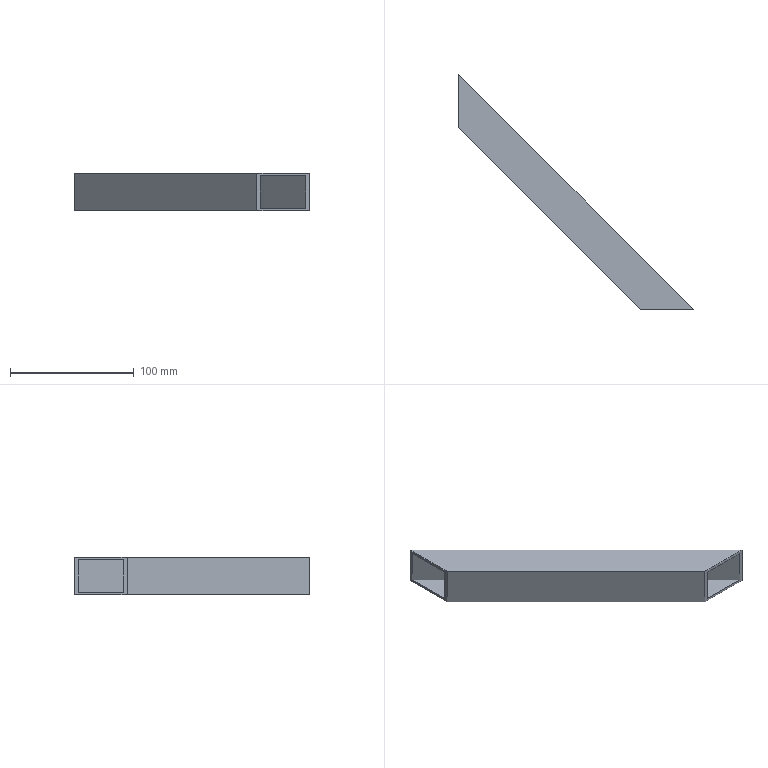Part | NX | features solid 2 | 1 solid | 10 faces | box 190 x 190 x 30 mm | volume 53469 mm3 | plane 10
STEP:
#1=CARTESIAN_POINT('',(380.,-462.426,-60.));
#2=VERTEX_POINT('',#1);
#3=CARTESIAN_POINT('',(380.,-420.,-60.));
#4=VERTEX_POINT('',#3);
#5=CARTESIAN_POINT('',(380.,-508.107,-60.));
#6=DIRECTION('',(0.,1.,0.));
#7=VECTOR('',#6,1000.);
#8=LINE('',#5,#7);
#9=EDGE_CURVE('',#2,#4,#8,.T.);
#10=ORIENTED_EDGE('',*,*,#9,.F.);
#11=CARTESIAN_POINT('',(380.,-462.426,-30.));
#12=VERTEX_POINT('',#11);
#13=CARTESIAN_POINT('',(380.,-462.426,-30.));
#14=DIRECTION('',(0.,0.,-1.));
#15=VECTOR('',#14,1000.);
#16=LINE('',#13,#15);
#17=EDGE_CURVE('',#12,#2,#16,.T.);
#18=ORIENTED_EDGE('',*,*,#17,.F.);
#19=CARTESIAN_POINT('',(380.,-420.,-30.));
#20=VERTEX_POINT('',#19);
#21=CARTESIAN_POINT('',(380.,-508.107,-30.));
#22=DIRECTION('',(0.,1.,0.));
#23=VECTOR('',#22,1000.);
#24=LINE('',#21,#23);
#25=EDGE_CURVE('',#12,#20,#24,.T.);
#26=ORIENTED_EDGE('',*,*,#25,.T.);
#27=CARTESIAN_POINT('',(380.,-420.,-30.));
#28=DIRECTION('',(0.,0.,-1.));
#29=VECTOR('',#28,1000.);
#30=LINE('',#27,#29);
#31=EDGE_CURVE('',#20,#4,#30,.T.);
#32=ORIENTED_EDGE('',*,*,#31,.T.);
#33=EDGE_LOOP('',(#10,#18,#26,#32));
#34=FACE_BOUND('',#33,.T.);
#35=CARTESIAN_POINT('',(380.,-459.598,-58.));
#36=VERTEX_POINT('',#35);
#37=CARTESIAN_POINT('',(380.,-422.828,-58.));
#38=VERTEX_POINT('',#37);
#39=CARTESIAN_POINT('',(380.,-508.107,-58.));
#40=DIRECTION('',(0.,1.,0.));
#41=VECTOR('',#40,1000.);
#42=LINE('',#39,#41);
#43=EDGE_CURVE('',#36,#38,#42,.T.);
#44=ORIENTED_EDGE('',*,*,#43,.T.);
#45=CARTESIAN_POINT('',(380.,-422.828,-32.));
#46=VERTEX_POINT('',#45);
#47=CARTESIAN_POINT('',(380.,-422.828,-30.));
#48=DIRECTION('',(0.,0.,-1.));
#49=VECTOR('',#48,1000.);
#50=LINE('',#47,#49);
#51=EDGE_CURVE('',#46,#38,#50,.T.);
#52=ORIENTED_EDGE('',*,*,#51,.F.);
#53=CARTESIAN_POINT('',(380.,-459.598,-32.));
#54=VERTEX_POINT('',#53);
#55=CARTESIAN_POINT('',(380.,-508.107,-32.));
#56=DIRECTION('',(0.,1.,0.));
#57=VECTOR('',#56,1000.);
#58=LINE('',#55,#57);
#59=EDGE_CURVE('',#54,#46,#58,.T.);
#60=ORIENTED_EDGE('',*,*,#59,.F.);
#61=CARTESIAN_POINT('',(380.,-459.598,-30.));
#62=DIRECTION('',(0.,0.,-1.));
#63=VECTOR('',#62,1000.);
#64=LINE('',#61,#63);
#65=EDGE_CURVE('',#54,#36,#64,.T.);
#66=ORIENTED_EDGE('',*,*,#65,.T.);
#67=EDGE_LOOP('',(#44,#52,#60,#66));
#68=FACE_BOUND('',#67,.T.);
#69=CARTESIAN_POINT('',(380.,-620.,-30.));
#70=DIRECTION('',(1.,0.,0.));
#71=DIRECTION('',(0.,0.,1.));
#72=AXIS2_PLACEMENT_3D('',#69,#70,#71);
#73=PLANE('',#72);
#74=ADVANCED_FACE('',(#34,#68),#73,.F.);
#75=CARTESIAN_POINT('',(570.,-610.,-60.));
#76=VERTEX_POINT('',#75);
#77=CARTESIAN_POINT('',(527.574,-610.,-60.));
#78=VERTEX_POINT('',#77);
#79=CARTESIAN_POINT('',(422.5,-610.,-60.));
#80=DIRECTION('',(-1.,0.,0.));
#81=VECTOR('',#80,1000.);
#82=LINE('',#79,#81);
#83=EDGE_CURVE('',#76,#78,#82,.T.);
#84=ORIENTED_EDGE('',*,*,#83,.F.);
#85=CARTESIAN_POINT('',(570.,-610.,-30.));
#86=VERTEX_POINT('',#85);
#87=CARTESIAN_POINT('',(570.,-610.,-30.));
#88=DIRECTION('',(0.,0.,-1.));
#89=VECTOR('',#88,1000.);
#90=LINE('',#87,#89);
#91=EDGE_CURVE('',#86,#76,#90,.T.);
#92=ORIENTED_EDGE('',*,*,#91,.F.);
#93=CARTESIAN_POINT('',(527.574,-610.,-30.));
#94=VERTEX_POINT('',#93);
#95=CARTESIAN_POINT('',(422.5,-610.,-30.));
#96=DIRECTION('',(-1.,0.,0.));
#97=VECTOR('',#96,1000.);
#98=LINE('',#95,#97);
#99=EDGE_CURVE('',#86,#94,#98,.T.);
#100=ORIENTED_EDGE('',*,*,#99,.T.);
#101=CARTESIAN_POINT('',(527.574,-610.,-30.));
#102=DIRECTION('',(0.,0.,-1.));
#103=VECTOR('',#102,1000.);
#104=LINE('',#101,#103);
#105=EDGE_CURVE('',#94,#78,#104,.T.);
#106=ORIENTED_EDGE('',*,*,#105,.T.);
#107=EDGE_LOOP('',(#84,#92,#100,#106));
#108=FACE_BOUND('',#107,.T.);
#109=CARTESIAN_POINT('',(567.172,-610.,-58.));
#110=VERTEX_POINT('',#109);
#111=CARTESIAN_POINT('',(530.402,-610.,-58.));
#112=VERTEX_POINT('',#111);
#113=CARTESIAN_POINT('',(422.5,-610.,-58.));
#114=DIRECTION('',(-1.,0.,0.));
#115=VECTOR('',#114,1000.);
#116=LINE('',#113,#115);
#117=EDGE_CURVE('',#110,#112,#116,.T.);
#118=ORIENTED_EDGE('',*,*,#117,.T.);
#119=CARTESIAN_POINT('',(530.402,-610.,-32.));
#120=VERTEX_POINT('',#119);
#121=CARTESIAN_POINT('',(530.402,-610.,-30.));
#122=DIRECTION('',(0.,0.,-1.));
#123=VECTOR('',#122,1000.);
#124=LINE('',#121,#123);
#125=EDGE_CURVE('',#120,#112,#124,.T.);
#126=ORIENTED_EDGE('',*,*,#125,.F.);
#127=CARTESIAN_POINT('',(567.172,-610.,-32.));
#128=VERTEX_POINT('',#127);
#129=CARTESIAN_POINT('',(422.5,-610.,-32.));
#130=DIRECTION('',(-1.,0.,0.));
#131=VECTOR('',#130,1000.);
#132=LINE('',#129,#131);
#133=EDGE_CURVE('',#128,#120,#132,.T.);
#134=ORIENTED_EDGE('',*,*,#133,.F.);
#135=CARTESIAN_POINT('',(567.172,-610.,-30.));
#136=DIRECTION('',(0.,0.,-1.));
#137=VECTOR('',#136,1000.);
#138=LINE('',#135,#137);
#139=EDGE_CURVE('',#128,#110,#138,.T.);
#140=ORIENTED_EDGE('',*,*,#139,.T.);
#141=EDGE_LOOP('',(#118,#126,#134,#140));
#142=FACE_BOUND('',#141,.T.);
#143=CARTESIAN_POINT('',(640.,-610.,-30.));
#144=DIRECTION('',(0.,1.,0.));
#145=DIRECTION('',(0.,0.,1.));
#146=AXIS2_PLACEMENT_3D('',#143,#144,#145);
#147=PLANE('',#146);
#148=ADVANCED_FACE('',(#108,#142),#147,.F.);
#149=CARTESIAN_POINT('',(350.,-390.,-60.));
#150=DIRECTION('',(0.7071,-0.7071,0.));
#151=VECTOR('',#150,1000.);
#152=LINE('',#149,#151);
#153=EDGE_CURVE('',#4,#76,#152,.T.);
#154=ORIENTED_EDGE('',*,*,#153,.F.);
#155=ORIENTED_EDGE('',*,*,#31,.F.);
#156=CARTESIAN_POINT('',(350.,-390.,-30.));
#157=DIRECTION('',(0.7071,-0.7071,0.));
#158=VECTOR('',#157,1000.);
#159=LINE('',#156,#158);
#160=EDGE_CURVE('',#20,#86,#159,.T.);
#161=ORIENTED_EDGE('',*,*,#160,.T.);
#162=ORIENTED_EDGE('',*,*,#91,.T.);
#163=EDGE_LOOP('',(#154,#155,#161,#162));
#164=FACE_BOUND('',#163,.T.);
#165=CARTESIAN_POINT('',(350.,-390.,-30.));
#166=DIRECTION('',(-0.7071,-0.7071,0.));
#167=DIRECTION('',(-0.7071,0.7071,0.));
#168=AXIS2_PLACEMENT_3D('',#165,#166,#167);
#169=PLANE('',#168);
#170=ADVANCED_FACE('',(#164),#169,.F.);
#171=CARTESIAN_POINT('',(350.,-432.426,-60.));
#172=DIRECTION('',(0.7071,-0.7071,0.));
#173=VECTOR('',#172,1000.);
#174=LINE('',#171,#173);
#175=EDGE_CURVE('',#2,#78,#174,.T.);
#176=ORIENTED_EDGE('',*,*,#175,.T.);
#177=ORIENTED_EDGE('',*,*,#105,.F.);
#178=CARTESIAN_POINT('',(350.,-432.426,-30.));
#179=DIRECTION('',(0.7071,-0.7071,0.));
#180=VECTOR('',#179,1000.);
#181=LINE('',#178,#180);
#182=EDGE_CURVE('',#12,#94,#181,.T.);
#183=ORIENTED_EDGE('',*,*,#182,.F.);
#184=ORIENTED_EDGE('',*,*,#17,.T.);
#185=EDGE_LOOP('',(#176,#177,#183,#184));
#186=FACE_BOUND('',#185,.T.);
#187=CARTESIAN_POINT('',(350.,-432.426,-30.));
#188=DIRECTION('',(-0.7071,-0.7071,0.));
#189=DIRECTION('',(-0.7071,0.7071,0.));
#190=AXIS2_PLACEMENT_3D('',#187,#188,#189);
#191=PLANE('',#190);
#192=ADVANCED_FACE('',(#186),#191,.T.);
#193=ORIENTED_EDGE('',*,*,#25,.F.);
#194=ORIENTED_EDGE('',*,*,#182,.T.);
#195=ORIENTED_EDGE('',*,*,#99,.F.);
#196=ORIENTED_EDGE('',*,*,#160,.F.);
#197=EDGE_LOOP('',(#193,#194,#195,#196));
#198=FACE_BOUND('',#197,.T.);
#199=CARTESIAN_POINT('',(422.5,-508.107,-30.));
#200=DIRECTION('',(0.,0.,1.));
#201=DIRECTION('',(-1.,0.,0.));
#202=AXIS2_PLACEMENT_3D('',#199,#200,#201);
#203=PLANE('',#202);
#204=ADVANCED_FACE('',(#198),#203,.T.);
#205=ORIENTED_EDGE('',*,*,#9,.T.);
#206=ORIENTED_EDGE('',*,*,#153,.T.);
#207=ORIENTED_EDGE('',*,*,#83,.T.);
#208=ORIENTED_EDGE('',*,*,#175,.F.);
#209=EDGE_LOOP('',(#205,#206,#207,#208));
#210=FACE_BOUND('',#209,.T.);
#211=CARTESIAN_POINT('',(422.5,-508.107,-60.));
#212=DIRECTION('',(0.,0.,1.));
#213=DIRECTION('',(-1.,0.,0.));
#214=AXIS2_PLACEMENT_3D('',#211,#212,#213);
#215=PLANE('',#214);
#216=ADVANCED_FACE('',(#210),#215,.F.);
#217=CARTESIAN_POINT('',(348.586,-391.414,-58.));
#218=DIRECTION('',(0.7071,-0.7071,0.));
#219=VECTOR('',#218,1000.);
#220=LINE('',#217,#219);
#221=EDGE_CURVE('',#38,#110,#220,.T.);
#222=ORIENTED_EDGE('',*,*,#221,.T.);
#223=ORIENTED_EDGE('',*,*,#139,.F.);
#224=CARTESIAN_POINT('',(348.586,-391.414,-32.));
#225=DIRECTION('',(0.7071,-0.7071,0.));
#226=VECTOR('',#225,1000.);
#227=LINE('',#224,#226);
#228=EDGE_CURVE('',#46,#128,#227,.T.);
#229=ORIENTED_EDGE('',*,*,#228,.F.);
#230=ORIENTED_EDGE('',*,*,#51,.T.);
#231=EDGE_LOOP('',(#222,#223,#229,#230));
#232=FACE_BOUND('',#231,.T.);
#233=CARTESIAN_POINT('',(348.586,-391.414,-30.));
#234=DIRECTION('',(-0.7071,-0.7071,0.));
#235=DIRECTION('',(-0.7071,0.7071,0.));
#236=AXIS2_PLACEMENT_3D('',#233,#234,#235);
#237=PLANE('',#236);
#238=ADVANCED_FACE('',(#232),#237,.T.);
#239=CARTESIAN_POINT('',(351.414,-431.012,-58.));
#240=DIRECTION('',(0.7071,-0.7071,0.));
#241=VECTOR('',#240,1000.);
#242=LINE('',#239,#241);
#243=EDGE_CURVE('',#36,#112,#242,.T.);
#244=ORIENTED_EDGE('',*,*,#243,.F.);
#245=ORIENTED_EDGE('',*,*,#65,.F.);
#246=CARTESIAN_POINT('',(351.414,-431.012,-32.));
#247=DIRECTION('',(0.7071,-0.7071,0.));
#248=VECTOR('',#247,1000.);
#249=LINE('',#246,#248);
#250=EDGE_CURVE('',#54,#120,#249,.T.);
#251=ORIENTED_EDGE('',*,*,#250,.T.);
#252=ORIENTED_EDGE('',*,*,#125,.T.);
#253=EDGE_LOOP('',(#244,#245,#251,#252));
#254=FACE_BOUND('',#253,.T.);
#255=CARTESIAN_POINT('',(351.414,-431.012,-30.));
#256=DIRECTION('',(-0.7071,-0.7071,0.));
#257=DIRECTION('',(-0.7071,0.7071,0.));
#258=AXIS2_PLACEMENT_3D('',#255,#256,#257);
#259=PLANE('',#258);
#260=ADVANCED_FACE('',(#254),#259,.F.);
#261=ORIENTED_EDGE('',*,*,#59,.T.);
#262=ORIENTED_EDGE('',*,*,#228,.T.);
#263=ORIENTED_EDGE('',*,*,#133,.T.);
#264=ORIENTED_EDGE('',*,*,#250,.F.);
#265=EDGE_LOOP('',(#261,#262,#263,#264));
#266=FACE_BOUND('',#265,.T.);
#267=CARTESIAN_POINT('',(422.5,-508.107,-32.));
#268=DIRECTION('',(0.,0.,1.));
#269=DIRECTION('',(-1.,0.,0.));
#270=AXIS2_PLACEMENT_3D('',#267,#268,#269);
#271=PLANE('',#270);
#272=ADVANCED_FACE('',(#266),#271,.F.);
#273=ORIENTED_EDGE('',*,*,#43,.F.);
#274=ORIENTED_EDGE('',*,*,#243,.T.);
#275=ORIENTED_EDGE('',*,*,#117,.F.);
#276=ORIENTED_EDGE('',*,*,#221,.F.);
#277=EDGE_LOOP('',(#273,#274,#275,#276));
#278=FACE_BOUND('',#277,.T.);
#279=CARTESIAN_POINT('',(422.5,-508.107,-58.));
#280=DIRECTION('',(0.,0.,1.));
#281=DIRECTION('',(-1.,0.,0.));
#282=AXIS2_PLACEMENT_3D('',#279,#280,#281);
#283=PLANE('',#282);
#284=ADVANCED_FACE('',(#278),#283,.T.);
#285=CLOSED_SHELL('',(#74,#148,#170,#192,#204,#216,#238,#260,#272,#284));
#286=MANIFOLD_SOLID_BREP('',#285);
#287=(LENGTH_UNIT()NAMED_UNIT(*)SI_UNIT(.MILLI.,.METRE.));
#288=UNCERTAINTY_MEASURE_WITH_UNIT(LENGTH_MEASURE(0.00001),#287,'','');
#289=(NAMED_UNIT(*)PLANE_ANGLE_UNIT()SI_UNIT($,.RADIAN.));
#290=(NAMED_UNIT(*)SI_UNIT($,.STERADIAN.)SOLID_ANGLE_UNIT());
#291=(GEOMETRIC_REPRESENTATION_CONTEXT(3)GLOBAL_UNCERTAINTY_ASSIGNED_CONTEXT((#288))GLOBAL_UNIT_ASSIGNED_CONTEXT((#287,#289,#290))REPRESENTATION_CONTEXT('',''));
#292=ADVANCED_BREP_SHAPE_REPRESENTATION('',(#286),#291);